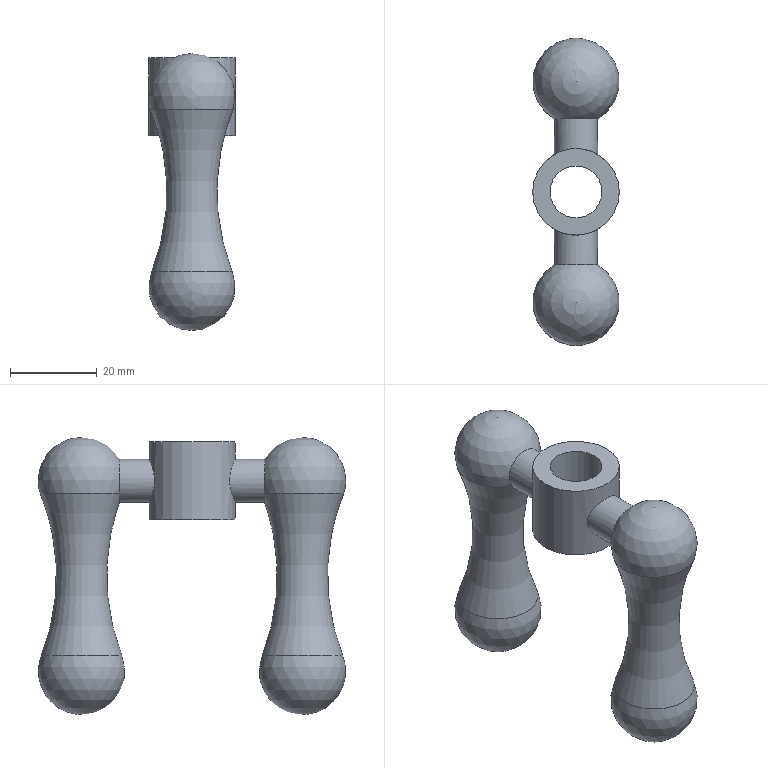Part | NX | features DATUM_CSYS 4, EXTRUDE 3, SKETCH 3, SWP104 2, UNITE 1 | 1 solid | 12 faces | box 20 x 71 x 64 mm | volume 28763 mm3 | cylinder 4 | sphere 4 | torus 2 | plane 2 | commonest cylinder face diameters 10 x2 12 x1 20 x1
STEP:
#1=CARTESIAN_POINT('',(0.,-10.,14.));
#2=VERTEX_POINT('',#1);
#3=CARTESIAN_POINT('',(-2.001,-9.858,13.723));
#4=CARTESIAN_POINT('',(0.6768,-10.148,14.276));
#5=CARTESIAN_POINT('',(3.912,-9.377,12.901));
#6=CARTESIAN_POINT('',(5.272,-8.49,9.69));
#7=CARTESIAN_POINT('',(4.729,-8.824,7.012));
#8=CARTESIAN_POINT('',(3.276,-9.538,4.841));
#9=CARTESIAN_POINT('',(0.01854,-10.309,3.449));
#10=CARTESIAN_POINT('',(-3.918,-9.379,5.086));
#11=CARTESIAN_POINT('',(-5.545,-8.305,8.981));
#12=CARTESIAN_POINT('',(-4.174,-9.187,12.262));
#13=CARTESIAN_POINT('',(-2.001,-9.858,13.723));
#14=CARTESIAN_POINT('',(0.6768,-10.148,14.276));
#15=CARTESIAN_POINT('',(3.912,-9.377,12.901));
#16=B_SPLINE_CURVE_WITH_KNOTS('',3,(#3,#4,#5,#6,#7,#8,#9,#10,#11,#12,#13,#14,#15),.UNSPECIFIED.,.T.,.F.,(1,1,1,1,1,1,1,1,1,1,1,1,1,1,1,1,1),(-0.007946,-0.003973,-0.001986,0.,0.003973,0.007946,0.009932,0.01192,0.01589,0.01986,0.02384,0.02781,0.0298,0.03178,0.03575,0.03973,0.04171),.UNSPECIFIED.);
#17=EDGE_CURVE('',#2,#2,#16,.T.);
#18=ORIENTED_EDGE('',*,*,#17,.F.);
#19=EDGE_LOOP('',(#18));
#20=FACE_BOUND('',#19,.T.);
#21=CARTESIAN_POINT('',(-4.099,-16.84,6.137));
#22=VERTEX_POINT('',#21);
#23=CARTESIAN_POINT('',(4.099,-16.84,6.137));
#24=VERTEX_POINT('',#23);
#25=CARTESIAN_POINT('',(-4.099,-16.84,6.137));
#26=CARTESIAN_POINT('',(-3.176,-17.006,4.815));
#27=CARTESIAN_POINT('',(-0.004214,-16.482,3.184));
#28=CARTESIAN_POINT('',(3.176,-17.006,4.816));
#29=CARTESIAN_POINT('',(4.099,-16.84,6.137));
#30=B_SPLINE_CURVE_WITH_KNOTS('',3,(#25,#26,#27,#28,#29),.UNSPECIFIED.,.F.,.F.,(4,1,4),(0.000000241,0.004784,0.009567),.UNSPECIFIED.);
#31=EDGE_CURVE('',#22,#24,#30,.T.);
#32=ORIENTED_EDGE('',*,*,#31,.F.);
#33=CARTESIAN_POINT('',(0.,-16.84,9.));
#34=DIRECTION('',(0.,-1.,0.));
#35=DIRECTION('',(0.,0.,-1.));
#36=AXIS2_PLACEMENT_3D('',#33,#34,#35);
#37=CIRCLE('',#36,5.);
#38=EDGE_CURVE('',#24,#22,#37,.T.);
#39=ORIENTED_EDGE('',*,*,#38,.F.);
#40=EDGE_LOOP('',(#32,#39));
#41=FACE_BOUND('',#40,.T.);
#42=CARTESIAN_POINT('',(0.,-18.,9.));
#43=DIRECTION('',(0.,1.,0.));
#44=DIRECTION('',(0.,0.,1.));
#45=AXIS2_PLACEMENT_3D('',#42,#43,#44);
#46=CYLINDRICAL_SURFACE('',#45,5.);
#47=ADVANCED_FACE('',(#20,#41),#46,.T.);
#48=CARTESIAN_POINT('',(4.099,16.84,6.137));
#49=VERTEX_POINT('',#48);
#50=CARTESIAN_POINT('',(-4.099,16.84,6.137));
#51=VERTEX_POINT('',#50);
#52=CARTESIAN_POINT('',(4.099,16.84,6.137));
#53=CARTESIAN_POINT('',(3.176,17.006,4.815));
#54=CARTESIAN_POINT('',(0.004214,16.482,3.184));
#55=CARTESIAN_POINT('',(-3.176,17.006,4.816));
#56=CARTESIAN_POINT('',(-4.099,16.84,6.137));
#57=B_SPLINE_CURVE_WITH_KNOTS('',3,(#52,#53,#54,#55,#56),.UNSPECIFIED.,.F.,.F.,(4,1,4),(0.000000241,0.004784,0.009567),.UNSPECIFIED.);
#58=EDGE_CURVE('',#49,#51,#57,.T.);
#59=ORIENTED_EDGE('',*,*,#58,.F.);
#60=CARTESIAN_POINT('',(0.,16.84,9.));
#61=DIRECTION('',(0.,1.,0.));
#62=DIRECTION('',(0.,0.,1.));
#63=AXIS2_PLACEMENT_3D('',#60,#61,#62);
#64=CIRCLE('',#63,5.);
#65=EDGE_CURVE('',#51,#49,#64,.T.);
#66=ORIENTED_EDGE('',*,*,#65,.F.);
#67=EDGE_LOOP('',(#59,#66));
#68=FACE_BOUND('',#67,.T.);
#69=CARTESIAN_POINT('',(0.,10.,14.));
#70=VERTEX_POINT('',#69);
#71=CARTESIAN_POINT('',(2.001,9.858,13.723));
#72=CARTESIAN_POINT('',(-0.6768,10.148,14.276));
#73=CARTESIAN_POINT('',(-3.912,9.377,12.901));
#74=CARTESIAN_POINT('',(-5.272,8.49,9.69));
#75=CARTESIAN_POINT('',(-4.729,8.824,7.012));
#76=CARTESIAN_POINT('',(-3.276,9.538,4.841));
#77=CARTESIAN_POINT('',(-0.01854,10.309,3.449));
#78=CARTESIAN_POINT('',(3.918,9.379,5.086));
#79=CARTESIAN_POINT('',(5.545,8.305,8.981));
#80=CARTESIAN_POINT('',(4.174,9.187,12.262));
#81=CARTESIAN_POINT('',(2.001,9.858,13.723));
#82=CARTESIAN_POINT('',(-0.6768,10.148,14.276));
#83=CARTESIAN_POINT('',(-3.912,9.377,12.901));
#84=B_SPLINE_CURVE_WITH_KNOTS('',3,(#71,#72,#73,#74,#75,#76,#77,#78,#79,#80,#81,#82,#83),.UNSPECIFIED.,.T.,.F.,(1,1,1,1,1,1,1,1,1,1,1,1,1,1,1,1,1),(-0.007946,-0.003973,-0.001986,0.,0.003973,0.007946,0.009932,0.01192,0.01589,0.01986,0.02384,0.02781,0.0298,0.03178,0.03575,0.03973,0.04171),.UNSPECIFIED.);
#85=EDGE_CURVE('',#70,#70,#84,.T.);
#86=ORIENTED_EDGE('',*,*,#85,.F.);
#87=EDGE_LOOP('',(#86));
#88=FACE_BOUND('',#87,.T.);
#89=CARTESIAN_POINT('',(0.,-18.,9.));
#90=DIRECTION('',(0.,1.,0.));
#91=DIRECTION('',(0.,0.,1.));
#92=AXIS2_PLACEMENT_3D('',#89,#90,#91);
#93=CYLINDRICAL_SURFACE('',#92,5.);
#94=ADVANCED_FACE('',(#68,#88),#93,.T.);
#95=CARTESIAN_POINT('',(-9.3,25.5,-31.324));
#96=VERTEX_POINT('',#95);
#97=CARTESIAN_POINT('',(0.,25.5,-31.324));
#98=DIRECTION('',(0.,0.,-1.));
#99=DIRECTION('',(-1.,0.,0.));
#100=AXIS2_PLACEMENT_3D('',#97,#98,#99);
#101=CIRCLE('',#100,9.3);
#102=EDGE_CURVE('',#96,#96,#101,.T.);
#103=ORIENTED_EDGE('',*,*,#102,.F.);
#104=EDGE_LOOP('',(#103));
#105=FACE_BOUND('',#104,.T.);
#106=CARTESIAN_POINT('',(0.,25.5,6.137));
#107=DIRECTION('',(0.,0.,-1.));
#108=DIRECTION('',(-1.,0.,0.));
#109=AXIS2_PLACEMENT_3D('',#106,#107,#108);
#110=CIRCLE('',#109,9.581);
#111=EDGE_CURVE('',#51,#49,#110,.T.);
#112=ORIENTED_EDGE('',*,*,#111,.T.);
#113=ORIENTED_EDGE('',*,*,#58,.T.);
#114=EDGE_LOOP('',(#112,#113));
#115=FACE_BOUND('',#114,.T.);
#116=CARTESIAN_POINT('',(0.,25.5,-12.942));
#117=DIRECTION('',(0.,0.,-1.));
#118=DIRECTION('',(-1.,0.,0.));
#119=AXIS2_PLACEMENT_3D('',#116,#117,#118);
#120=TOROIDAL_SURFACE('',#119,55.798,50.);
#121=ADVANCED_FACE('',(#105,#115),#120,.F.);
#122=ORIENTED_EDGE('',*,*,#111,.F.);
#123=ORIENTED_EDGE('',*,*,#65,.T.);
#124=EDGE_LOOP('',(#122,#123));
#125=FACE_BOUND('',#124,.T.);
#126=CARTESIAN_POINT('',(0.,25.5,9.));
#127=DIRECTION('',(0.,0.,-1.));
#128=DIRECTION('',(0.,1.,0.));
#129=AXIS2_PLACEMENT_3D('',#126,#127,#128);
#130=SPHERICAL_SURFACE('',#129,10.);
#131=ADVANCED_FACE('',(#125),#130,.T.);
#132=ORIENTED_EDGE('',*,*,#102,.T.);
#133=EDGE_LOOP('',(#132));
#134=FACE_BOUND('',#133,.T.);
#135=CARTESIAN_POINT('',(0.,25.5,-35.));
#136=DIRECTION('',(0.,0.,-1.));
#137=DIRECTION('',(0.,1.,0.));
#138=AXIS2_PLACEMENT_3D('',#135,#136,#137);
#139=SPHERICAL_SURFACE('',#138,10.);
#140=ADVANCED_FACE('',(#134),#139,.T.);
#141=ORIENTED_EDGE('',*,*,#85,.T.);
#142=EDGE_LOOP('',(#141));
#143=FACE_BOUND('',#142,.T.);
#144=CARTESIAN_POINT('',(10.,0.,18.));
#145=VERTEX_POINT('',#144);
#146=CARTESIAN_POINT('',(0.,0.,18.));
#147=DIRECTION('',(0.,0.,1.));
#148=DIRECTION('',(1.,0.,0.));
#149=AXIS2_PLACEMENT_3D('',#146,#147,#148);
#150=CIRCLE('',#149,10.);
#151=EDGE_CURVE('',#145,#145,#150,.T.);
#152=ORIENTED_EDGE('',*,*,#151,.F.);
#153=EDGE_LOOP('',(#152));
#154=FACE_BOUND('',#153,.T.);
#155=CARTESIAN_POINT('',(10.,0.,0.));
#156=VERTEX_POINT('',#155);
#157=CARTESIAN_POINT('',(0.,0.,0.));
#158=DIRECTION('',(0.,0.,1.));
#159=DIRECTION('',(1.,0.,0.));
#160=AXIS2_PLACEMENT_3D('',#157,#158,#159);
#161=CIRCLE('',#160,10.);
#162=EDGE_CURVE('',#156,#156,#161,.T.);
#163=ORIENTED_EDGE('',*,*,#162,.T.);
#164=EDGE_LOOP('',(#163));
#165=FACE_BOUND('',#164,.T.);
#166=ORIENTED_EDGE('',*,*,#17,.T.);
#167=EDGE_LOOP('',(#166));
#168=FACE_BOUND('',#167,.T.);
#169=CARTESIAN_POINT('',(0.,0.,18.));
#170=DIRECTION('',(0.,0.,-1.));
#171=DIRECTION('',(-1.,0.,0.));
#172=AXIS2_PLACEMENT_3D('',#169,#170,#171);
#173=CYLINDRICAL_SURFACE('',#172,10.);
#174=ADVANCED_FACE('',(#143,#154,#165,#168),#173,.T.);
#175=CARTESIAN_POINT('',(6.,0.,18.));
#176=VERTEX_POINT('',#175);
#177=CARTESIAN_POINT('',(0.,0.,18.));
#178=DIRECTION('',(0.,0.,1.));
#179=DIRECTION('',(1.,0.,0.));
#180=AXIS2_PLACEMENT_3D('',#177,#178,#179);
#181=CIRCLE('',#180,6.);
#182=EDGE_CURVE('',#176,#176,#181,.T.);
#183=ORIENTED_EDGE('',*,*,#182,.T.);
#184=EDGE_LOOP('',(#183));
#185=FACE_BOUND('',#184,.T.);
#186=CARTESIAN_POINT('',(6.,0.,0.));
#187=VERTEX_POINT('',#186);
#188=CARTESIAN_POINT('',(0.,0.,0.));
#189=DIRECTION('',(0.,0.,1.));
#190=DIRECTION('',(1.,0.,0.));
#191=AXIS2_PLACEMENT_3D('',#188,#189,#190);
#192=CIRCLE('',#191,6.);
#193=EDGE_CURVE('',#187,#187,#192,.T.);
#194=ORIENTED_EDGE('',*,*,#193,.F.);
#195=EDGE_LOOP('',(#194));
#196=FACE_BOUND('',#195,.T.);
#197=CARTESIAN_POINT('',(0.,0.,18.));
#198=DIRECTION('',(0.,0.,-1.));
#199=DIRECTION('',(-1.,0.,0.));
#200=AXIS2_PLACEMENT_3D('',#197,#198,#199);
#201=CYLINDRICAL_SURFACE('',#200,6.);
#202=ADVANCED_FACE('',(#185,#196),#201,.F.);
#203=ORIENTED_EDGE('',*,*,#151,.T.);
#204=EDGE_LOOP('',(#203));
#205=FACE_BOUND('',#204,.T.);
#206=ORIENTED_EDGE('',*,*,#182,.F.);
#207=EDGE_LOOP('',(#206));
#208=FACE_BOUND('',#207,.T.);
#209=CARTESIAN_POINT('',(0.,0.,18.));
#210=DIRECTION('',(0.,0.,1.));
#211=DIRECTION('',(1.,0.,0.));
#212=AXIS2_PLACEMENT_3D('',#209,#210,#211);
#213=PLANE('',#212);
#214=ADVANCED_FACE('',(#205,#208),#213,.T.);
#215=ORIENTED_EDGE('',*,*,#162,.F.);
#216=EDGE_LOOP('',(#215));
#217=FACE_BOUND('',#216,.T.);
#218=ORIENTED_EDGE('',*,*,#193,.T.);
#219=EDGE_LOOP('',(#218));
#220=FACE_BOUND('',#219,.T.);
#221=CARTESIAN_POINT('',(0.,0.,0.));
#222=DIRECTION('',(0.,0.,1.));
#223=DIRECTION('',(1.,0.,0.));
#224=AXIS2_PLACEMENT_3D('',#221,#222,#223);
#225=PLANE('',#224);
#226=ADVANCED_FACE('',(#217,#220),#225,.F.);
#227=CARTESIAN_POINT('',(-9.3,-25.5,-31.324));
#228=VERTEX_POINT('',#227);
#229=CARTESIAN_POINT('',(0.,-25.5,-31.324));
#230=DIRECTION('',(0.,0.,-1.));
#231=DIRECTION('',(-1.,0.,0.));
#232=AXIS2_PLACEMENT_3D('',#229,#230,#231);
#233=CIRCLE('',#232,9.3);
#234=EDGE_CURVE('',#228,#228,#233,.T.);
#235=ORIENTED_EDGE('',*,*,#234,.F.);
#236=EDGE_LOOP('',(#235));
#237=FACE_BOUND('',#236,.T.);
#238=CARTESIAN_POINT('',(0.,-25.5,6.137));
#239=DIRECTION('',(0.,0.,-1.));
#240=DIRECTION('',(-1.,0.,0.));
#241=AXIS2_PLACEMENT_3D('',#238,#239,#240);
#242=CIRCLE('',#241,9.581);
#243=EDGE_CURVE('',#24,#22,#242,.T.);
#244=ORIENTED_EDGE('',*,*,#243,.T.);
#245=ORIENTED_EDGE('',*,*,#31,.T.);
#246=EDGE_LOOP('',(#244,#245));
#247=FACE_BOUND('',#246,.T.);
#248=CARTESIAN_POINT('',(0.,-25.5,-12.942));
#249=DIRECTION('',(0.,0.,-1.));
#250=DIRECTION('',(-1.,0.,0.));
#251=AXIS2_PLACEMENT_3D('',#248,#249,#250);
#252=TOROIDAL_SURFACE('',#251,55.798,50.);
#253=ADVANCED_FACE('',(#237,#247),#252,.F.);
#254=ORIENTED_EDGE('',*,*,#243,.F.);
#255=ORIENTED_EDGE('',*,*,#38,.T.);
#256=EDGE_LOOP('',(#254,#255));
#257=FACE_BOUND('',#256,.T.);
#258=CARTESIAN_POINT('',(0.,-25.5,9.));
#259=DIRECTION('',(0.,0.,-1.));
#260=DIRECTION('',(0.,-1.,0.));
#261=AXIS2_PLACEMENT_3D('',#258,#259,#260);
#262=SPHERICAL_SURFACE('',#261,10.);
#263=ADVANCED_FACE('',(#257),#262,.T.);
#264=ORIENTED_EDGE('',*,*,#234,.T.);
#265=EDGE_LOOP('',(#264));
#266=FACE_BOUND('',#265,.T.);
#267=CARTESIAN_POINT('',(0.,-25.5,-35.));
#268=DIRECTION('',(0.,0.,-1.));
#269=DIRECTION('',(0.,-1.,0.));
#270=AXIS2_PLACEMENT_3D('',#267,#268,#269);
#271=SPHERICAL_SURFACE('',#270,10.);
#272=ADVANCED_FACE('',(#266),#271,.T.);
#273=CLOSED_SHELL('',(#47,#94,#121,#131,#140,#174,#202,#214,#226,#253,#263,#272));
#274=MANIFOLD_SOLID_BREP('',#273);
#275=(LENGTH_UNIT()NAMED_UNIT(*)SI_UNIT(.MILLI.,.METRE.));
#276=UNCERTAINTY_MEASURE_WITH_UNIT(LENGTH_MEASURE(0.0508),#275,'','');
#277=(NAMED_UNIT(*)PLANE_ANGLE_UNIT()SI_UNIT($,.RADIAN.));
#278=(NAMED_UNIT(*)SI_UNIT($,.STERADIAN.)SOLID_ANGLE_UNIT());
#279=(GEOMETRIC_REPRESENTATION_CONTEXT(3)GLOBAL_UNCERTAINTY_ASSIGNED_CONTEXT((#276))GLOBAL_UNIT_ASSIGNED_CONTEXT((#275,#277,#278))REPRESENTATION_CONTEXT('',''));
#280=ADVANCED_BREP_SHAPE_REPRESENTATION('',(#274),#279);